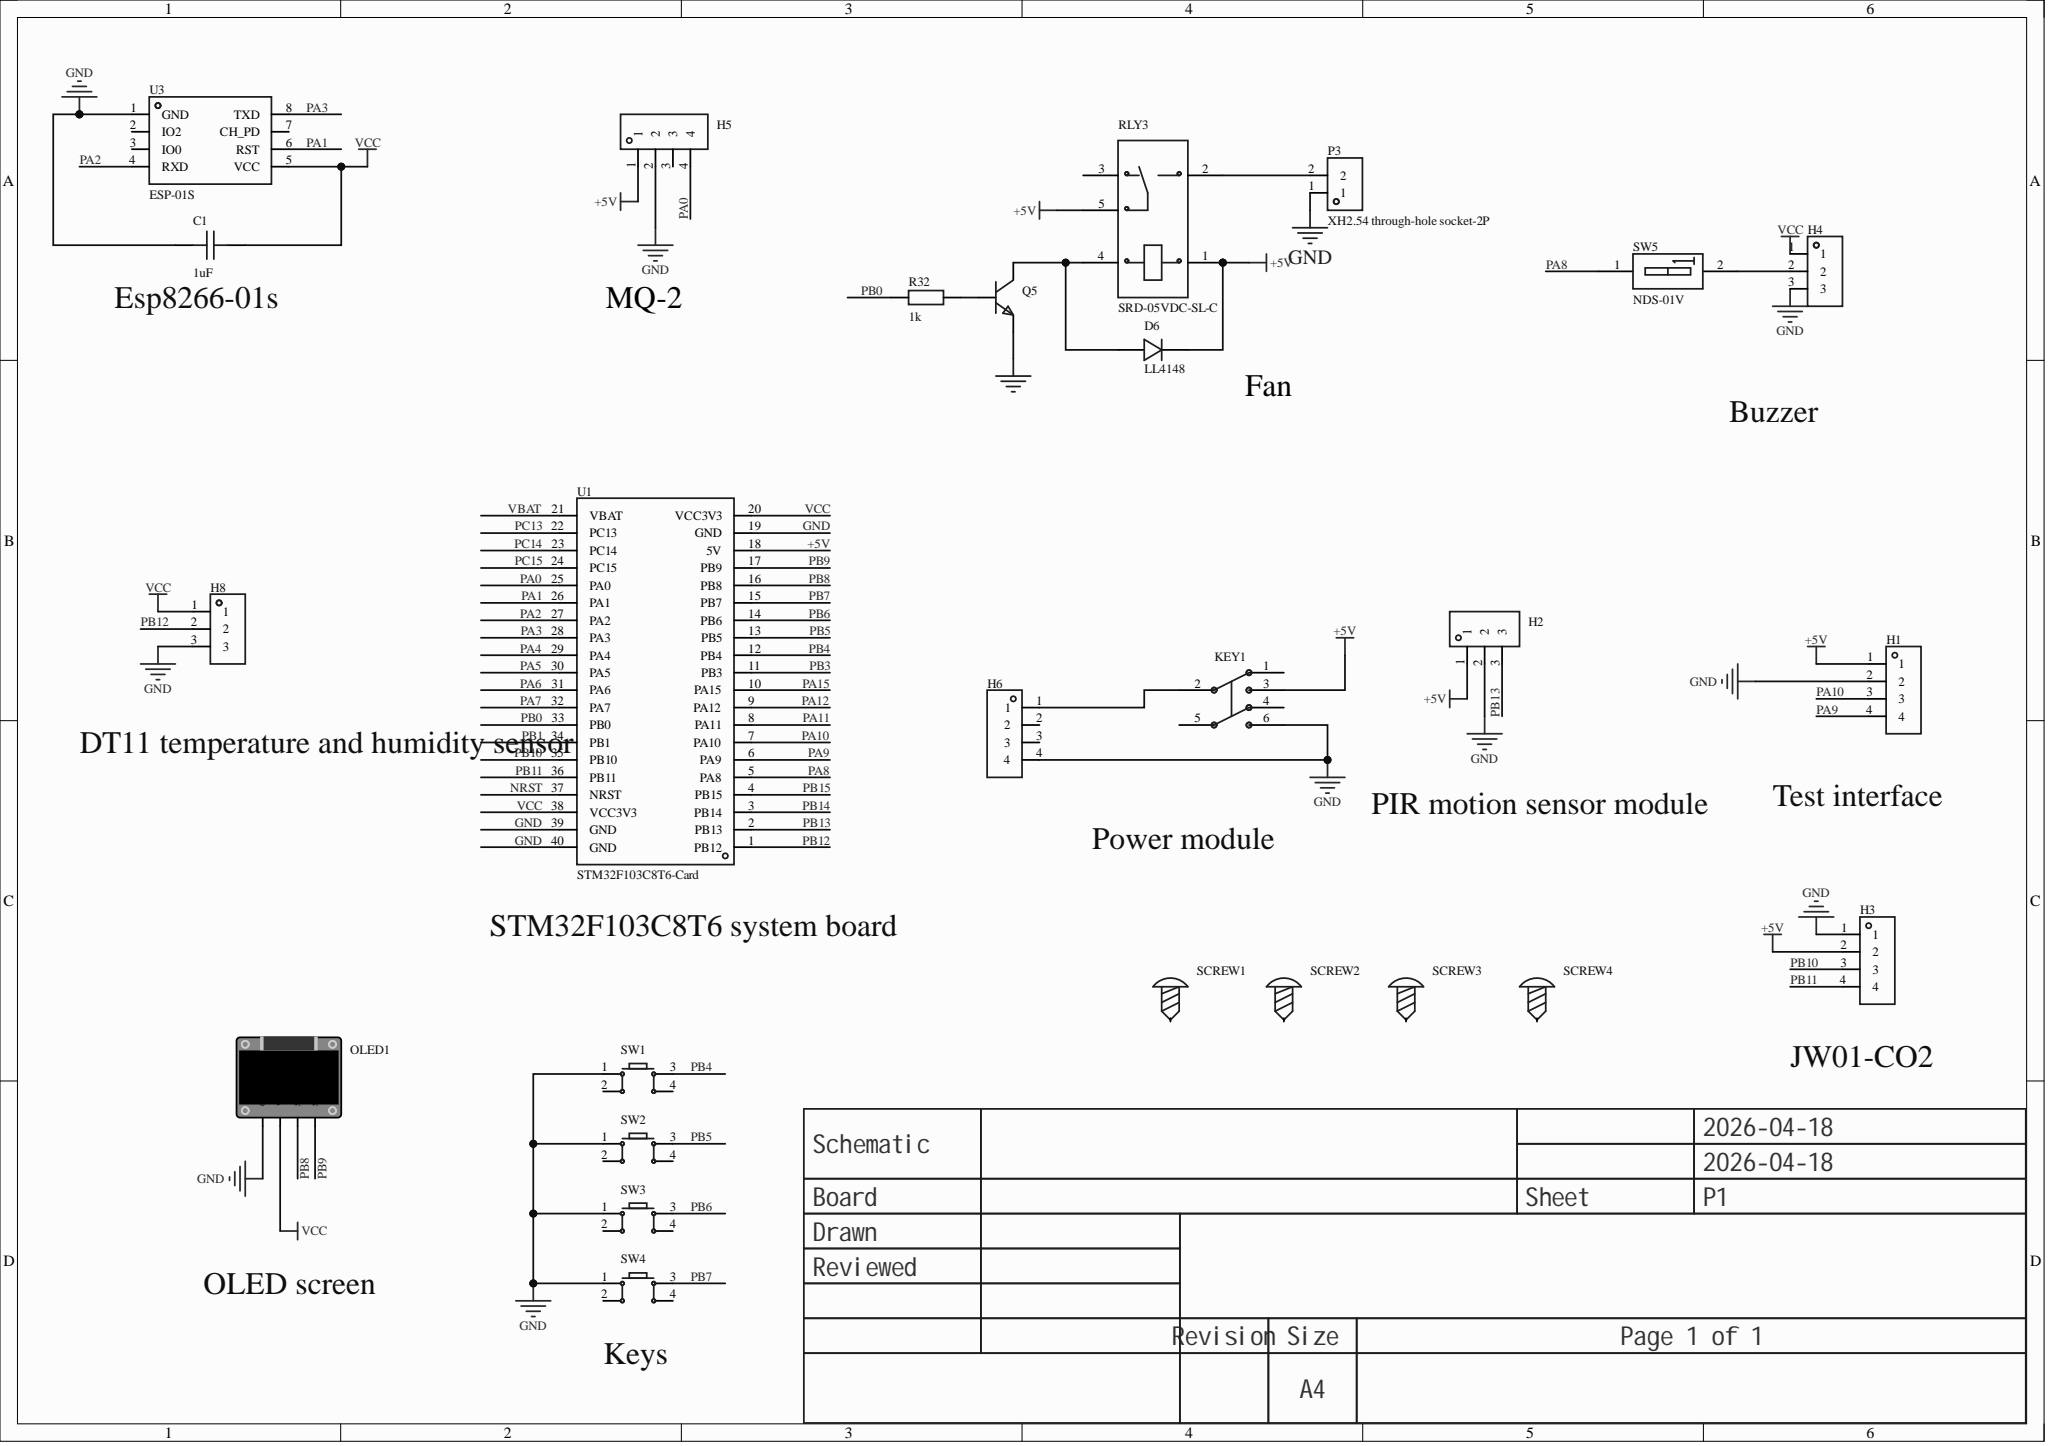Circuit board | Altium Designer | 26 parts | 26 nets
Bill of materials:
Comment,Description,Designator,Footprint,LibRef,Quantity
"1uF","","C1","C0603","CAP_0603","1"
"LL4148","二极管配置:-;功率:500mW;直流反向耐压(Vr):75V;平均整流电流(Io):200mA;正向压降(Vf):1V@10mA;反向电流(Ir):5uA@75V;反向恢复时间(trr):4ns;工作温度:+175℃@(Tj);","D6","LL-34_L3.5-W1.5-RD","LL4148_C9808","1"
"","","H1, H3","HDR-TH_4P-P2.54-V-M","HDR-M_2.54_1x4P","2"
"","","H2, H4, H8","HDR-TH_3P-P2.54-V-F","HDR-F_2.54_1x3P","3"
"","","H5, H6","HDR-TH_4P-P2.54-V-F","HDR-F_2.54_1x4P","2"
"Non-latching switch 8.5×8.5 silent","6 pins, 8.5×8.5","KEY1","SW-TH_6P-L8.5-W8.5-P2.54","无自锁开关 8.5×8.5 无声","1"
"","","OLED1","0.96OLED_4P","0.96OLED模块_4P","1"
"XH2.54 through-hole socket-2P","","P3","CONN-TH_XH2.54-2P","XH2.54直插座-2P","1"
"","","Q5","S8050_SOT-23","S8050_SOT_NPN","1"
"1k","","R32","R0603","Res_0603","1"
"SRD-05VDC-SL-C","Coil voltage:5V;Contact form:1C (SPDT) changeover;Contact capacity (resistive load):-;Max switching voltage:250V@AC;Max switching current:15A;","RLY3","RELAY-TH_SRD-XXVDC-XL-C","SRD-05VDC-SL-C","1"
"","","SCREW1, SCREW2, SCREW3, SCREW4","M3螺丝","M3螺丝","4"
"","","SW1, SW2, SW3, SW4","SW-TH_4P-L6.0-W6.0-P4.50-LS6.5","Key_TH_6x6x6","4"
"NDS-01V","Forward-action high lever","SW5","SW-TH_2P-L3.9-W9.9-P2.54-LS7.6","NDS-01V_C501305","1"
"STM32F103C8T6-Card","","U1","CONN-TH_L53.3-W22.9_STM32F103C8T6-CARD","STM32F103C8T6-Card","1"
"ESP-01S","","U3","WIFIM-TH_ESP-01S","ESP-01S_C111009","1"
Netlist (Protel format):
[
C1
C0603
1uF



]
[
D6
LL-34_L3.5-W1.5-RD
LL4148



]
[
H1
HDR-TH_4P-P2.54-V-M




]
[
H2
HDR-TH_3P-P2.54-V-F




]
[
H3
HDR-TH_4P-P2.54-V-M




]
[
H4
HDR-TH_3P-P2.54-V-F




]
[
H5
HDR-TH_4P-P2.54-V-F




]
[
H6
HDR-TH_4P-P2.54-V-F




]
[
H8
HDR-TH_3P-P2.54-V-F




]
[
KEY1
SW-TH_6P-L8.5-W8.5-P2.54
Non-latching switch 8.5×8.5 silent



]
[
OLED1
0.96OLED_4P




]
[
P3
CONN-TH_XH2.54-2P
XH2.54 through-hole socket-2P



]
[
Q5
S8050_SOT-23




]
[
R32
R0603
1k



]
[
RLY3
RELAY-TH_SRD-XXVDC-XL-C
SRD-05VDC-SL-C



]
[
SCREW1
M3螺丝




]
[
SCREW2
M3螺丝




]
[
SCREW3
M3螺丝




]
[
SCREW4
M3螺丝




]
[
SW1
SW-TH_4P-L6.0-W6.0-P4.50-LS6.5




]
[
SW2
SW-TH_4P-L6.0-W6.0-P4.50-LS6.5




]
[
SW3
SW-TH_4P-L6.0-W6.0-P4.50-LS6.5




]
[
SW4
SW-TH_4P-L6.0-W6.0-P4.50-LS6.5




]
[
SW5
SW-TH_2P-L3.9-W9.9-P2.54-LS7.6
NDS-01V



]
[
U1
CONN-TH_L53.3-W22.9_STM32F103C8T6-CARD
STM32F103C8T6-Card



]
[
U3
WIFIM-TH_ESP-01S
ESP-01S



]
(
VCC
C1-2
H4-1
H8-1
OLED1-2
U1-20
U1-38
U3-5
)
(
PB13
H2-3
U1-2
)
(
PB12
H8-2
U1-1
)
(
PB11
H3-4
U1-36
)
(
PB10
H3-3
U1-35
)
(
PB9
OLED1-4
U1-17
)
(
PB8
OLED1-3
U1-16
)
(
PB7
SW4-3
U1-15
)
(
PB6
SW3-3
U1-14
)
(
PB5
SW2-3
U1-13
)
(
PB4
SW1-3
U1-12
)
(
PB0
R32-1
U1-33
)
(
PA10
H1-3
U1-7
)
(
PA9
H1-4
U1-6
)
(
PA8
SW5-1
U1-5
)
(
PA3
U1-28
U3-8
)
(
PA2
U1-27
U3-4
)
(
PA1
U1-26
U3-6
)
(
PA0
H5-4
U1-25
)
(
NetQ5_1
Q5-1
R32-2
)
(
NetP3_2
P3-2
RLY3-2
)
(
NetH6_1
H6-1
KEY1-2
)
(
NetH4_2
H4-2
SW5-2
)
(
NetD6_2
D6-2
Q5-3
RLY3-4
)
(
GND
C1-1
H1-2
H2-2
H3-1
H4-3
H5-2
H6-4
H8-3
KEY1-6
OLED1-1
P3-1
Q5-2
SW1-1
SW2-1
SW3-1
SW4-1
U1-19
U1-39
U1-40
U3-1
)
(
+5V
D6-1
H1-1
H2-1
H3-2
H5-1
KEY1-3
RLY3-1
RLY3-5
U1-18
)